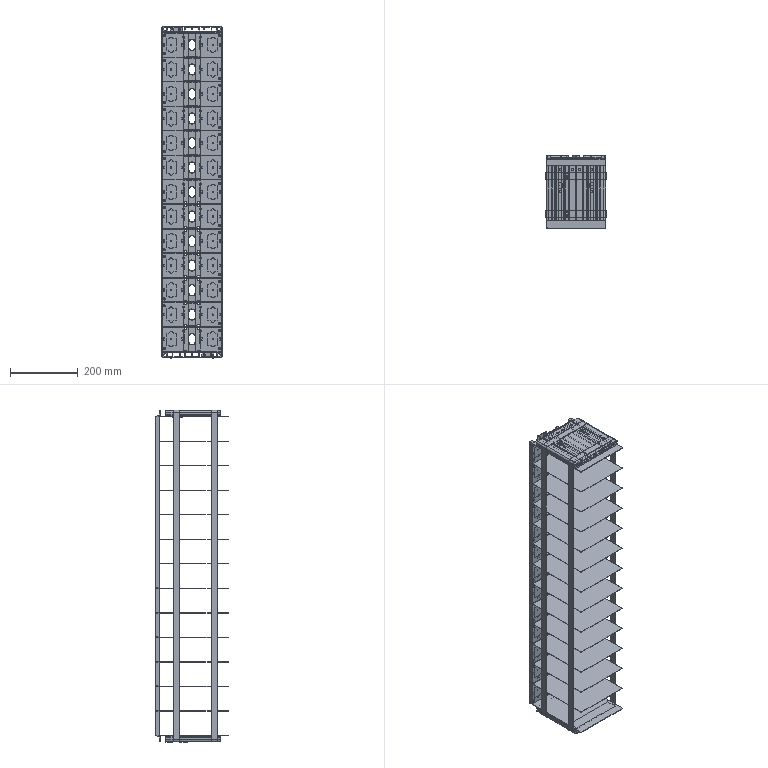Part | NX | features BREP 10 | 38 solids | 5112 faces | volume 1550668 mm3 | plane 2946 | cylinder 2166 | commonest cylinder face diameters 2 x433 4 x402 3 x208 6 x178 0.6 x164 10 x108